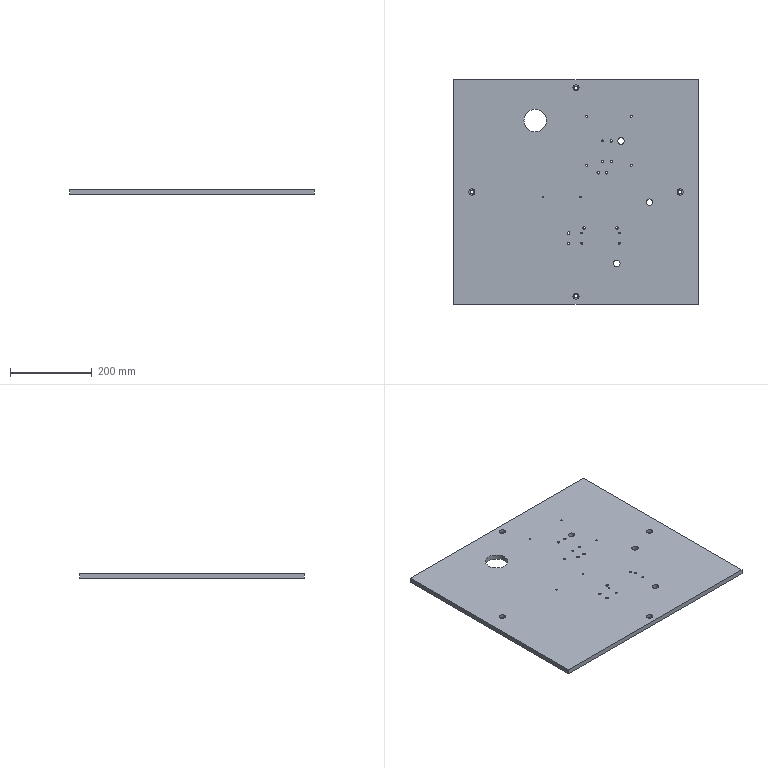Part | NX | features BREP 1 | 1 solid | 78 faces | box 600 x 550 x 12 mm | volume 3912725 mm3 | cylinder 64 | plane 10 | cone 4 | commonest cylinder face diameters 4.2 x16 6 x16 8.4 x8 15 x8 16 x6 3.3 x4